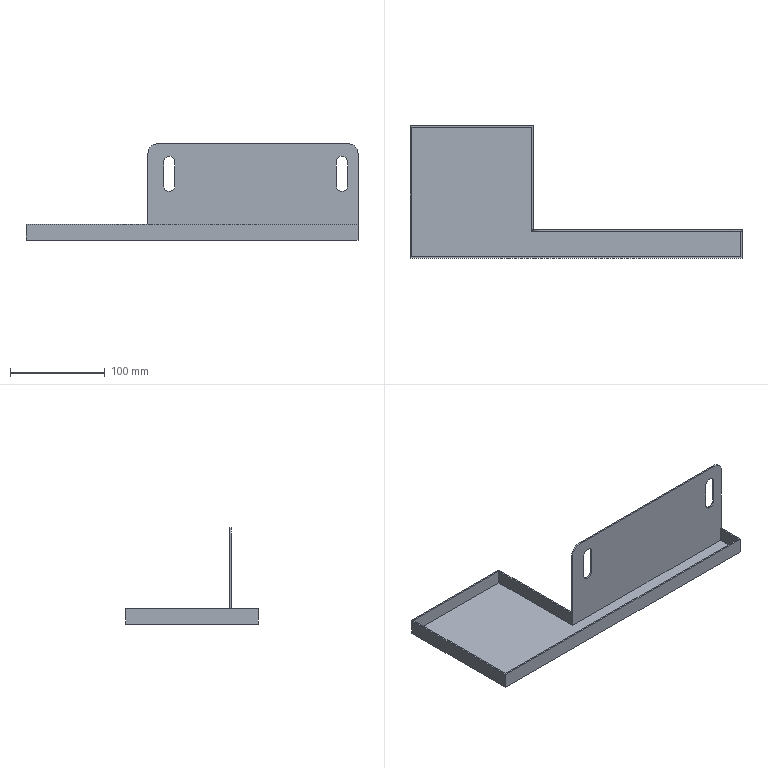Part | SolidWorks | features ICE 3, BossThin 1, Extrusion 1, Fillet 1 | 1 solid | 28 faces | box 350 x 140 x 101.5 mm | volume 86053 mm3 | plane 20 | cylinder 8 | commonest cylinder face diameters 12 x6 20 x2
STEP:
#1=CARTESIAN_POINT('',(-24.,-40.,51.5));
#2=VERTEX_POINT('',#1);
#3=CARTESIAN_POINT('',(-18.,-40.,57.5));
#4=VERTEX_POINT('',#3);
#5=CARTESIAN_POINT('',(-24.,-40.,57.5));
#6=DIRECTION('',(0.,-1.,0.));
#7=DIRECTION('',(1.,0.,0.));
#8=AXIS2_PLACEMENT_3D('',#5,#6,#7);
#9=CIRCLE('',#8,6.);
#10=EDGE_CURVE('',#2,#4,#9,.T.);
#11=ORIENTED_EDGE('',*,*,#10,.F.);
#12=CARTESIAN_POINT('',(-24.,-41.5,51.5));
#13=VERTEX_POINT('',#12);
#14=CARTESIAN_POINT('',(-24.,58.5,51.5));
#15=DIRECTION('',(0.,-1.,0.));
#16=VECTOR('',#15,1000.);
#17=LINE('',#14,#16);
#18=EDGE_CURVE('',#2,#13,#17,.T.);
#19=ORIENTED_EDGE('',*,*,#18,.T.);
#20=CARTESIAN_POINT('',(-18.,-41.5,57.5));
#21=VERTEX_POINT('',#20);
#22=CARTESIAN_POINT('',(-24.,-41.5,57.5));
#23=DIRECTION('',(0.,-1.,0.));
#24=DIRECTION('',(0.,0.,-1.));
#25=AXIS2_PLACEMENT_3D('',#22,#23,#24);
#26=CIRCLE('',#25,6.);
#27=EDGE_CURVE('',#13,#21,#26,.T.);
#28=ORIENTED_EDGE('',*,*,#27,.T.);
#29=CARTESIAN_POINT('',(-18.,58.5,57.5));
#30=DIRECTION('',(0.,-1.,0.));
#31=VECTOR('',#30,1000.);
#32=LINE('',#29,#31);
#33=EDGE_CURVE('',#4,#21,#32,.T.);
#34=ORIENTED_EDGE('',*,*,#33,.F.);
#35=EDGE_LOOP('',(#11,#19,#28,#34));
#36=FACE_OUTER_BOUND('',#35,.T.);
#37=CARTESIAN_POINT('',(-24.,58.5,57.5));
#38=DIRECTION('',(0.,-1.,0.));
#39=DIRECTION('',(0.,0.,-1.));
#40=AXIS2_PLACEMENT_3D('',#37,#38,#39);
#41=CYLINDRICAL_SURFACE('',#40,6.);
#42=ADVANCED_FACE('',(#36),#41,.F.);
#43=CARTESIAN_POINT('',(158.,-40.,51.5));
#44=VERTEX_POINT('',#43);
#45=CARTESIAN_POINT('',(164.,-40.,57.5));
#46=VERTEX_POINT('',#45);
#47=CARTESIAN_POINT('',(158.,-40.,57.5));
#48=DIRECTION('',(0.,-1.,0.));
#49=DIRECTION('',(1.,0.,0.));
#50=AXIS2_PLACEMENT_3D('',#47,#48,#49);
#51=CIRCLE('',#50,6.);
#52=EDGE_CURVE('',#44,#46,#51,.T.);
#53=ORIENTED_EDGE('',*,*,#52,.F.);
#54=CARTESIAN_POINT('',(158.,-41.5,51.5));
#55=VERTEX_POINT('',#54);
#56=CARTESIAN_POINT('',(158.,58.5,51.5));
#57=DIRECTION('',(0.,-1.,0.));
#58=VECTOR('',#57,1000.);
#59=LINE('',#56,#58);
#60=EDGE_CURVE('',#44,#55,#59,.T.);
#61=ORIENTED_EDGE('',*,*,#60,.T.);
#62=CARTESIAN_POINT('',(164.,-41.5,57.5));
#63=VERTEX_POINT('',#62);
#64=CARTESIAN_POINT('',(158.,-41.5,57.5));
#65=DIRECTION('',(0.,-1.,0.));
#66=DIRECTION('',(0.,0.,-1.));
#67=AXIS2_PLACEMENT_3D('',#64,#65,#66);
#68=CIRCLE('',#67,6.);
#69=EDGE_CURVE('',#55,#63,#68,.T.);
#70=ORIENTED_EDGE('',*,*,#69,.T.);
#71=CARTESIAN_POINT('',(164.,58.5,57.5));
#72=DIRECTION('',(0.,-1.,0.));
#73=VECTOR('',#72,1000.);
#74=LINE('',#71,#73);
#75=EDGE_CURVE('',#46,#63,#74,.T.);
#76=ORIENTED_EDGE('',*,*,#75,.F.);
#77=EDGE_LOOP('',(#53,#61,#70,#76));
#78=FACE_OUTER_BOUND('',#77,.T.);
#79=CARTESIAN_POINT('',(158.,58.5,57.5));
#80=DIRECTION('',(0.,-1.,0.));
#81=DIRECTION('',(0.,0.,-1.));
#82=AXIS2_PLACEMENT_3D('',#79,#80,#81);
#83=CYLINDRICAL_SURFACE('',#82,6.);
#84=ADVANCED_FACE('',(#78),#83,.F.);
#85=CARTESIAN_POINT('',(-46.5,-41.5,1.5));
#86=VERTEX_POINT('',#85);
#87=CARTESIAN_POINT('',(173.5,-41.5,1.5));
#88=VERTEX_POINT('',#87);
#89=CARTESIAN_POINT('',(-46.5,-41.5,1.5));
#90=DIRECTION('',(1.,0.,0.));
#91=VECTOR('',#90,1000.);
#92=LINE('',#89,#91);
#93=EDGE_CURVE('',#86,#88,#92,.T.);
#94=ORIENTED_EDGE('',*,*,#93,.F.);
#95=CARTESIAN_POINT('',(-46.5,68.5,1.5));
#96=VERTEX_POINT('',#95);
#97=CARTESIAN_POINT('',(-46.5,70.,1.5));
#98=DIRECTION('',(0.,1.,0.));
#99=VECTOR('',#98,1000.);
#100=LINE('',#97,#99);
#101=EDGE_CURVE('',#86,#96,#100,.T.);
#102=ORIENTED_EDGE('',*,*,#101,.T.);
#103=CARTESIAN_POINT('',(-173.5,68.5,1.5));
#104=VERTEX_POINT('',#103);
#105=CARTESIAN_POINT('',(-45.,68.5,1.5));
#106=DIRECTION('',(-1.,0.,0.));
#107=VECTOR('',#106,1000.);
#108=LINE('',#105,#107);
#109=EDGE_CURVE('',#96,#104,#108,.T.);
#110=ORIENTED_EDGE('',*,*,#109,.T.);
#111=CARTESIAN_POINT('',(-173.5,-68.5,1.5));
#112=VERTEX_POINT('',#111);
#113=CARTESIAN_POINT('',(-173.5,70.,1.5));
#114=DIRECTION('',(0.,-1.,0.));
#115=VECTOR('',#114,1000.);
#116=LINE('',#113,#115);
#117=EDGE_CURVE('',#104,#112,#116,.T.);
#118=ORIENTED_EDGE('',*,*,#117,.T.);
#119=CARTESIAN_POINT('',(173.5,-68.5,1.5));
#120=VERTEX_POINT('',#119);
#121=CARTESIAN_POINT('',(-175.,-68.5,1.5));
#122=DIRECTION('',(1.,0.,0.));
#123=VECTOR('',#122,1000.);
#124=LINE('',#121,#123);
#125=EDGE_CURVE('',#112,#120,#124,.T.);
#126=ORIENTED_EDGE('',*,*,#125,.T.);
#127=CARTESIAN_POINT('',(173.5,-70.,1.5));
#128=DIRECTION('',(0.,1.,0.));
#129=VECTOR('',#128,1000.);
#130=LINE('',#127,#129);
#131=EDGE_CURVE('',#120,#88,#130,.T.);
#132=ORIENTED_EDGE('',*,*,#131,.T.);
#133=EDGE_LOOP('',(#94,#102,#110,#118,#126,#132));
#134=FACE_OUTER_BOUND('',#133,.T.);
#135=CARTESIAN_POINT('',(0.,0.,1.5));
#136=DIRECTION('',(0.,0.,1.));
#137=DIRECTION('',(1.,0.,0.));
#138=AXIS2_PLACEMENT_3D('',#135,#136,#137);
#139=PLANE('',#138);
#140=ADVANCED_FACE('',(#134),#139,.T.);
#141=CARTESIAN_POINT('',(173.5,-68.5,16.5));
#142=VERTEX_POINT('',#141);
#143=CARTESIAN_POINT('',(173.5,-41.5,16.5));
#144=VERTEX_POINT('',#143);
#145=CARTESIAN_POINT('',(173.5,-70.,16.5));
#146=DIRECTION('',(0.,1.,0.));
#147=VECTOR('',#146,1000.);
#148=LINE('',#145,#147);
#149=EDGE_CURVE('',#142,#144,#148,.T.);
#150=ORIENTED_EDGE('',*,*,#149,.T.);
#151=CARTESIAN_POINT('',(173.5,-41.5,16.5));
#152=DIRECTION('',(0.,0.,-1.));
#153=VECTOR('',#152,1000.);
#154=LINE('',#151,#153);
#155=EDGE_CURVE('',#144,#88,#154,.T.);
#156=ORIENTED_EDGE('',*,*,#155,.T.);
#157=ORIENTED_EDGE('',*,*,#131,.F.);
#158=CARTESIAN_POINT('',(173.5,-68.5,16.5));
#159=DIRECTION('',(0.,0.,-1.));
#160=VECTOR('',#159,1000.);
#161=LINE('',#158,#160);
#162=EDGE_CURVE('',#142,#120,#161,.T.);
#163=ORIENTED_EDGE('',*,*,#162,.F.);
#164=EDGE_LOOP('',(#150,#156,#157,#163));
#165=FACE_OUTER_BOUND('',#164,.T.);
#166=CARTESIAN_POINT('',(173.5,-70.,16.5));
#167=DIRECTION('',(-1.,0.,0.));
#168=DIRECTION('',(0.,0.,1.));
#169=AXIS2_PLACEMENT_3D('',#166,#167,#168);
#170=PLANE('',#169);
#171=ADVANCED_FACE('',(#165),#170,.T.);
#172=CARTESIAN_POINT('',(175.,-41.5,16.5));
#173=VERTEX_POINT('',#172);
#174=CARTESIAN_POINT('',(0.,-41.5,16.5));
#175=DIRECTION('',(1.,0.,0.));
#176=VECTOR('',#175,1000.);
#177=LINE('',#174,#176);
#178=EDGE_CURVE('',#144,#173,#177,.T.);
#179=ORIENTED_EDGE('',*,*,#178,.F.);
#180=ORIENTED_EDGE('',*,*,#149,.F.);
#181=CARTESIAN_POINT('',(-173.5,-68.5,16.5));
#182=VERTEX_POINT('',#181);
#183=CARTESIAN_POINT('',(-175.,-68.5,16.5));
#184=DIRECTION('',(1.,0.,0.));
#185=VECTOR('',#184,1000.);
#186=LINE('',#183,#185);
#187=EDGE_CURVE('',#182,#142,#186,.T.);
#188=ORIENTED_EDGE('',*,*,#187,.F.);
#189=CARTESIAN_POINT('',(-173.5,68.5,16.5));
#190=VERTEX_POINT('',#189);
#191=CARTESIAN_POINT('',(-173.5,70.,16.5));
#192=DIRECTION('',(0.,-1.,0.));
#193=VECTOR('',#192,1000.);
#194=LINE('',#191,#193);
#195=EDGE_CURVE('',#190,#182,#194,.T.);
#196=ORIENTED_EDGE('',*,*,#195,.F.);
#197=CARTESIAN_POINT('',(-46.5,68.5,16.5));
#198=VERTEX_POINT('',#197);
#199=CARTESIAN_POINT('',(-45.,68.5,16.5));
#200=DIRECTION('',(-1.,0.,0.));
#201=VECTOR('',#200,1000.);
#202=LINE('',#199,#201);
#203=EDGE_CURVE('',#198,#190,#202,.T.);
#204=ORIENTED_EDGE('',*,*,#203,.F.);
#205=CARTESIAN_POINT('',(-46.5,-40.,16.5));
#206=VERTEX_POINT('',#205);
#207=CARTESIAN_POINT('',(-46.5,70.,16.5));
#208=DIRECTION('',(0.,1.,0.));
#209=VECTOR('',#208,1000.);
#210=LINE('',#207,#209);
#211=EDGE_CURVE('',#206,#198,#210,.T.);
#212=ORIENTED_EDGE('',*,*,#211,.F.);
#213=CARTESIAN_POINT('',(-45.,-40.,16.5));
#214=VERTEX_POINT('',#213);
#215=CARTESIAN_POINT('',(-45.,-40.,16.5));
#216=DIRECTION('',(-1.,0.,0.));
#217=VECTOR('',#216,1000.);
#218=LINE('',#215,#217);
#219=EDGE_CURVE('',#214,#206,#218,.T.);
#220=ORIENTED_EDGE('',*,*,#219,.F.);
#221=CARTESIAN_POINT('',(-45.,70.,16.5));
#222=VERTEX_POINT('',#221);
#223=CARTESIAN_POINT('',(-45.,70.,16.5));
#224=DIRECTION('',(0.,1.,0.));
#225=VECTOR('',#224,1000.);
#226=LINE('',#223,#225);
#227=EDGE_CURVE('',#214,#222,#226,.T.);
#228=ORIENTED_EDGE('',*,*,#227,.T.);
#229=CARTESIAN_POINT('',(-175.,70.,16.5));
#230=VERTEX_POINT('',#229);
#231=CARTESIAN_POINT('',(-45.,70.,16.5));
#232=DIRECTION('',(-1.,0.,0.));
#233=VECTOR('',#232,1000.);
#234=LINE('',#231,#233);
#235=EDGE_CURVE('',#222,#230,#234,.T.);
#236=ORIENTED_EDGE('',*,*,#235,.T.);
#237=CARTESIAN_POINT('',(-175.,-70.,16.5));
#238=VERTEX_POINT('',#237);
#239=CARTESIAN_POINT('',(-175.,70.,16.5));
#240=DIRECTION('',(0.,-1.,0.));
#241=VECTOR('',#240,1000.);
#242=LINE('',#239,#241);
#243=EDGE_CURVE('',#230,#238,#242,.T.);
#244=ORIENTED_EDGE('',*,*,#243,.T.);
#245=CARTESIAN_POINT('',(175.,-70.,16.5));
#246=VERTEX_POINT('',#245);
#247=CARTESIAN_POINT('',(-175.,-70.,16.5));
#248=DIRECTION('',(1.,0.,0.));
#249=VECTOR('',#248,1000.);
#250=LINE('',#247,#249);
#251=EDGE_CURVE('',#238,#246,#250,.T.);
#252=ORIENTED_EDGE('',*,*,#251,.T.);
#253=CARTESIAN_POINT('',(175.,-70.,16.5));
#254=DIRECTION('',(0.,1.,0.));
#255=VECTOR('',#254,1000.);
#256=LINE('',#253,#255);
#257=EDGE_CURVE('',#246,#173,#256,.T.);
#258=ORIENTED_EDGE('',*,*,#257,.T.);
#259=EDGE_LOOP('',(#179,#180,#188,#196,#204,#212,#220,#228,#236,#244,#252,#258));
#260=FACE_OUTER_BOUND('',#259,.T.);
#261=CARTESIAN_POINT('',(0.,0.,16.5));
#262=DIRECTION('',(0.,0.,-1.));
#263=DIRECTION('',(-1.,0.,0.));
#264=AXIS2_PLACEMENT_3D('',#261,#262,#263);
#265=PLANE('',#264);
#266=ADVANCED_FACE('',(#260),#265,.F.);
#267=CARTESIAN_POINT('',(175.,-40.,0.));
#268=VERTEX_POINT('',#267);
#269=CARTESIAN_POINT('',(175.,-40.,91.5));
#270=VERTEX_POINT('',#269);
#271=CARTESIAN_POINT('',(175.,-40.,-0.5));
#272=DIRECTION('',(0.,0.,1.));
#273=VECTOR('',#272,1000.);
#274=LINE('',#271,#273);
#275=EDGE_CURVE('',#268,#270,#274,.T.);
#276=ORIENTED_EDGE('',*,*,#275,.T.);
#277=CARTESIAN_POINT('',(175.,-41.5,91.5));
#278=VERTEX_POINT('',#277);
#279=CARTESIAN_POINT('',(175.,-41.5,91.5));
#280=DIRECTION('',(0.,-1.,0.));
#281=VECTOR('',#280,1000.);
#282=LINE('',#279,#281);
#283=EDGE_CURVE('',#270,#278,#282,.T.);
#284=ORIENTED_EDGE('',*,*,#283,.T.);
#285=CARTESIAN_POINT('',(175.,-41.5,101.5));
#286=DIRECTION('',(0.,0.,-1.));
#287=VECTOR('',#286,1000.);
#288=LINE('',#285,#287);
#289=EDGE_CURVE('',#278,#173,#288,.T.);
#290=ORIENTED_EDGE('',*,*,#289,.T.);
#291=ORIENTED_EDGE('',*,*,#257,.F.);
#292=CARTESIAN_POINT('',(175.,-70.,0.));
#293=VERTEX_POINT('',#292);
#294=CARTESIAN_POINT('',(175.,-70.,1.5));
#295=DIRECTION('',(0.,0.,-1.));
#296=VECTOR('',#295,1000.);
#297=LINE('',#294,#296);
#298=EDGE_CURVE('',#246,#293,#297,.T.);
#299=ORIENTED_EDGE('',*,*,#298,.T.);
#300=CARTESIAN_POINT('',(175.,70.,0.));
#301=DIRECTION('',(0.,1.,0.));
#302=VECTOR('',#301,1000.);
#303=LINE('',#300,#302);
#304=EDGE_CURVE('',#293,#268,#303,.T.);
#305=ORIENTED_EDGE('',*,*,#304,.T.);
#306=EDGE_LOOP('',(#276,#284,#290,#291,#299,#305));
#307=FACE_OUTER_BOUND('',#306,.T.);
#308=CARTESIAN_POINT('',(175.,70.,1.5));
#309=DIRECTION('',(-1.,0.,0.));
#310=DIRECTION('',(0.,0.,1.));
#311=AXIS2_PLACEMENT_3D('',#308,#309,#310);
#312=PLANE('',#311);
#313=ADVANCED_FACE('',(#307),#312,.F.);
#314=CARTESIAN_POINT('',(-175.,70.,0.));
#315=VERTEX_POINT('',#314);
#316=CARTESIAN_POINT('',(-175.,70.,1.5));
#317=DIRECTION('',(0.,0.,-1.));
#318=VECTOR('',#317,1000.);
#319=LINE('',#316,#318);
#320=EDGE_CURVE('',#230,#315,#319,.T.);
#321=ORIENTED_EDGE('',*,*,#320,.F.);
#322=ORIENTED_EDGE('',*,*,#235,.F.);
#323=CARTESIAN_POINT('',(-45.,70.,0.));
#324=VERTEX_POINT('',#323);
#325=CARTESIAN_POINT('',(-45.,70.,-0.5));
#326=DIRECTION('',(0.,0.,1.));
#327=VECTOR('',#326,1000.);
#328=LINE('',#325,#327);
#329=EDGE_CURVE('',#324,#222,#328,.T.);
#330=ORIENTED_EDGE('',*,*,#329,.F.);
#331=CARTESIAN_POINT('',(-175.,70.,0.));
#332=DIRECTION('',(-1.,0.,0.));
#333=VECTOR('',#332,1000.);
#334=LINE('',#331,#333);
#335=EDGE_CURVE('',#324,#315,#334,.T.);
#336=ORIENTED_EDGE('',*,*,#335,.T.);
#337=EDGE_LOOP('',(#321,#322,#330,#336));
#338=FACE_OUTER_BOUND('',#337,.T.);
#339=CARTESIAN_POINT('',(-175.,70.,1.5));
#340=DIRECTION('',(0.,-1.,0.));
#341=DIRECTION('',(0.,0.,-1.));
#342=AXIS2_PLACEMENT_3D('',#339,#340,#341);
#343=PLANE('',#342);
#344=ADVANCED_FACE('',(#338),#343,.F.);
#345=CARTESIAN_POINT('',(-175.,-70.,0.));
#346=VERTEX_POINT('',#345);
#347=CARTESIAN_POINT('',(-175.,70.,0.));
#348=DIRECTION('',(0.,-1.,0.));
#349=VECTOR('',#348,1000.);
#350=LINE('',#347,#349);
#351=EDGE_CURVE('',#315,#346,#350,.T.);
#352=ORIENTED_EDGE('',*,*,#351,.T.);
#353=CARTESIAN_POINT('',(-175.,-70.,1.5));
#354=DIRECTION('',(0.,0.,-1.));
#355=VECTOR('',#354,1000.);
#356=LINE('',#353,#355);
#357=EDGE_CURVE('',#238,#346,#356,.T.);
#358=ORIENTED_EDGE('',*,*,#357,.F.);
#359=ORIENTED_EDGE('',*,*,#243,.F.);
#360=ORIENTED_EDGE('',*,*,#320,.T.);
#361=EDGE_LOOP('',(#352,#358,#359,#360));
#362=FACE_OUTER_BOUND('',#361,.T.);
#363=CARTESIAN_POINT('',(-175.,70.,1.5));
#364=DIRECTION('',(1.,0.,0.));
#365=DIRECTION('',(0.,0.,-1.));
#366=AXIS2_PLACEMENT_3D('',#363,#364,#365);
#367=PLANE('',#366);
#368=ADVANCED_FACE('',(#362),#367,.F.);
#369=CARTESIAN_POINT('',(-175.,-70.,0.));
#370=DIRECTION('',(1.,0.,0.));
#371=VECTOR('',#370,1000.);
#372=LINE('',#369,#371);
#373=EDGE_CURVE('',#346,#293,#372,.T.);
#374=ORIENTED_EDGE('',*,*,#373,.T.);
#375=ORIENTED_EDGE('',*,*,#298,.F.);
#376=ORIENTED_EDGE('',*,*,#251,.F.);
#377=ORIENTED_EDGE('',*,*,#357,.T.);
#378=EDGE_LOOP('',(#374,#375,#376,#377));
#379=FACE_OUTER_BOUND('',#378,.T.);
#380=CARTESIAN_POINT('',(-175.,-70.,1.5));
#381=DIRECTION('',(0.,1.,0.));
#382=DIRECTION('',(0.,0.,1.));
#383=AXIS2_PLACEMENT_3D('',#380,#381,#382);
#384=PLANE('',#383);
#385=ADVANCED_FACE('',(#379),#384,.F.);
#386=CARTESIAN_POINT('',(-45.,-40.,0.));
#387=VERTEX_POINT('',#386);
#388=CARTESIAN_POINT('',(-45.,0.,0.));
#389=DIRECTION('',(0.,-1.,0.));
#390=VECTOR('',#389,1000.);
#391=LINE('',#388,#390);
#392=EDGE_CURVE('',#324,#387,#391,.T.);
#393=ORIENTED_EDGE('',*,*,#392,.T.);
#394=CARTESIAN_POINT('',(0.,-40.,0.));
#395=DIRECTION('',(1.,0.,0.));
#396=VECTOR('',#395,1000.);
#397=LINE('',#394,#396);
#398=EDGE_CURVE('',#387,#268,#397,.T.);
#399=ORIENTED_EDGE('',*,*,#398,.T.);
#400=ORIENTED_EDGE('',*,*,#304,.F.);
#401=ORIENTED_EDGE('',*,*,#373,.F.);
#402=ORIENTED_EDGE('',*,*,#351,.F.);
#403=ORIENTED_EDGE('',*,*,#335,.F.);
#404=EDGE_LOOP('',(#393,#399,#400,#401,#402,#403));
#405=FACE_OUTER_BOUND('',#404,.T.);
#406=CARTESIAN_POINT('',(0.,0.,0.));
#407=DIRECTION('',(0.,0.,1.));
#408=DIRECTION('',(1.,0.,0.));
#409=AXIS2_PLACEMENT_3D('',#406,#407,#408);
#410=PLANE('',#409);
#411=ADVANCED_FACE('',(#405),#410,.F.);
#412=CARTESIAN_POINT('',(-18.,-40.,82.5));
#413=VERTEX_POINT('',#412);
#414=CARTESIAN_POINT('',(-18.,-40.,-0.5));
#415=DIRECTION('',(0.,0.,1.));
#416=VECTOR('',#415,1000.);
#417=LINE('',#414,#416);
#418=EDGE_CURVE('',#4,#413,#417,.T.);
#419=ORIENTED_EDGE('',*,*,#418,.T.);
#420=CARTESIAN_POINT('',(-30.,-40.,82.5));
#421=VERTEX_POINT('',#420);
#422=CARTESIAN_POINT('',(-24.,-40.,82.5));
#423=DIRECTION('',(0.,-1.,0.));
#424=DIRECTION('',(1.,0.,0.));
#425=AXIS2_PLACEMENT_3D('',#422,#423,#424);
#426=CIRCLE('',#425,6.);
#427=EDGE_CURVE('',#413,#421,#426,.T.);
#428=ORIENTED_EDGE('',*,*,#427,.T.);
#429=CARTESIAN_POINT('',(-30.,-40.,57.5));
#430=VERTEX_POINT('',#429);
#431=CARTESIAN_POINT('',(-30.,-40.,-0.5));
#432=DIRECTION('',(0.,0.,-1.));
#433=VECTOR('',#432,1000.);
#434=LINE('',#431,#433);
#435=EDGE_CURVE('',#421,#430,#434,.T.);
#436=ORIENTED_EDGE('',*,*,#435,.T.);
#437=CARTESIAN_POINT('',(-24.,-40.,57.5));
#438=DIRECTION('',(0.,-1.,0.));
#439=DIRECTION('',(1.,0.,0.));
#440=AXIS2_PLACEMENT_3D('',#437,#438,#439);
#441=CIRCLE('',#440,6.);
#442=EDGE_CURVE('',#430,#2,#441,.T.);
#443=ORIENTED_EDGE('',*,*,#442,.T.);
#444=ORIENTED_EDGE('',*,*,#10,.T.);
#445=EDGE_LOOP('',(#419,#428,#436,#443,#444));
#446=FACE_BOUND('',#445,.T.);
#447=CARTESIAN_POINT('',(164.,-40.,82.5));
#448=VERTEX_POINT('',#447);
#449=CARTESIAN_POINT('',(164.,-40.,-0.5));
#450=DIRECTION('',(0.,0.,1.));
#451=VECTOR('',#450,1000.);
#452=LINE('',#449,#451);
#453=EDGE_CURVE('',#46,#448,#452,.T.);
#454=ORIENTED_EDGE('',*,*,#453,.T.);
#455=CARTESIAN_POINT('',(152.,-40.,82.5));
#456=VERTEX_POINT('',#455);
#457=CARTESIAN_POINT('',(158.,-40.,82.5));
#458=DIRECTION('',(0.,-1.,0.));
#459=DIRECTION('',(1.,0.,0.));
#460=AXIS2_PLACEMENT_3D('',#457,#458,#459);
#461=CIRCLE('',#460,6.);
#462=EDGE_CURVE('',#448,#456,#461,.T.);
#463=ORIENTED_EDGE('',*,*,#462,.T.);
#464=CARTESIAN_POINT('',(152.,-40.,57.5));
#465=VERTEX_POINT('',#464);
#466=CARTESIAN_POINT('',(152.,-40.,-0.5));
#467=DIRECTION('',(0.,0.,-1.));
#468=VECTOR('',#467,1000.);
#469=LINE('',#466,#468);
#470=EDGE_CURVE('',#456,#465,#469,.T.);
#471=ORIENTED_EDGE('',*,*,#470,.T.);
#472=CARTESIAN_POINT('',(158.,-40.,57.5));
#473=DIRECTION('',(0.,-1.,0.));
#474=DIRECTION('',(1.,0.,0.));
#475=AXIS2_PLACEMENT_3D('',#472,#473,#474);
#476=CIRCLE('',#475,6.);
#477=EDGE_CURVE('',#465,#44,#476,.T.);
#478=ORIENTED_EDGE('',*,*,#477,.T.);
#479=ORIENTED_EDGE('',*,*,#52,.T.);
#480=EDGE_LOOP('',(#454,#463,#471,#478,#479));
#481=FACE_BOUND('',#480,.T.);
#482=CARTESIAN_POINT('',(165.,-40.,101.5));
#483=VERTEX_POINT('',#482);
#484=CARTESIAN_POINT('',(-36.5,-40.,101.5));
#485=VERTEX_POINT('',#484);
#486=CARTESIAN_POINT('',(-46.5,-40.,101.5));
#487=DIRECTION('',(-1.,0.,0.));
#488=VECTOR('',#487,1000.);
#489=LINE('',#486,#488);
#490=EDGE_CURVE('',#483,#485,#489,.T.);
#491=ORIENTED_EDGE('',*,*,#490,.F.);
#492=CARTESIAN_POINT('',(165.,-40.,91.5));
#493=DIRECTION('',(0.,1.,0.));
#494=DIRECTION('',(1.,0.,0.));
#495=AXIS2_PLACEMENT_3D('',#492,#493,#494);
#496=CIRCLE('',#495,10.);
#497=EDGE_CURVE('',#483,#270,#496,.T.);
#498=ORIENTED_EDGE('',*,*,#497,.T.);
#499=ORIENTED_EDGE('',*,*,#275,.F.);
#500=ORIENTED_EDGE('',*,*,#398,.F.);
#501=CARTESIAN_POINT('',(-45.,-40.,-0.5));
#502=DIRECTION('',(0.,0.,1.));
#503=VECTOR('',#502,1000.);
#504=LINE('',#501,#503);
#505=EDGE_CURVE('',#387,#214,#504,.T.);
#506=ORIENTED_EDGE('',*,*,#505,.T.);
#507=ORIENTED_EDGE('',*,*,#219,.T.);
#508=CARTESIAN_POINT('',(-46.5,-40.,91.5));
#509=VERTEX_POINT('',#508);
#510=CARTESIAN_POINT('',(-46.5,-40.,101.5));
#511=DIRECTION('',(0.,0.,-1.));
#512=VECTOR('',#511,1000.);
#513=LINE('',#510,#512);
#514=EDGE_CURVE('',#509,#206,#513,.T.);
#515=ORIENTED_EDGE('',*,*,#514,.F.);
#516=CARTESIAN_POINT('',(-36.5,-40.,91.5));
#517=DIRECTION('',(0.,1.,0.));
#518=DIRECTION('',(1.,0.,0.));
#519=AXIS2_PLACEMENT_3D('',#516,#517,#518);
#520=CIRCLE('',#519,10.);
#521=EDGE_CURVE('',#509,#485,#520,.T.);
#522=ORIENTED_EDGE('',*,*,#521,.T.);
#523=EDGE_LOOP('',(#491,#498,#499,#500,#506,#507,#515,#522));
#524=FACE_OUTER_BOUND('',#523,.T.);
#525=CARTESIAN_POINT('',(175.,-40.,-0.5));
#526=DIRECTION('',(0.,-1.,0.));
#527=DIRECTION('',(1.,0.,0.));
#528=AXIS2_PLACEMENT_3D('',#525,#526,#527);
#529=PLANE('',#528);
#530=ADVANCED_FACE('',(#446,#481,#524),#529,.F.);
#531=ORIENTED_EDGE('',*,*,#329,.T.);
#532=ORIENTED_EDGE('',*,*,#227,.F.);
#533=ORIENTED_EDGE('',*,*,#505,.F.);
#534=ORIENTED_EDGE('',*,*,#392,.F.);
#535=EDGE_LOOP('',(#531,#532,#533,#534));
#536=FACE_OUTER_BOUND('',#535,.T.);
#537=CARTESIAN_POINT('',(-45.,70.,-0.5));
#538=DIRECTION('',(-1.,0.,0.));
#539=DIRECTION('',(0.,-1.,0.));
#540=AXIS2_PLACEMENT_3D('',#537,#538,#539);
#541=PLANE('',#540);
#542=ADVANCED_FACE('',(#536),#541,.F.);
#543=ORIENTED_EDGE('',*,*,#125,.F.);
#544=CARTESIAN_POINT('',(-173.5,-68.5,16.5));
#545=DIRECTION('',(0.,0.,-1.));
#546=VECTOR('',#545,1000.);
#547=LINE('',#544,#546);
#548=EDGE_CURVE('',#182,#112,#547,.T.);
#549=ORIENTED_EDGE('',*,*,#548,.F.);
#550=ORIENTED_EDGE('',*,*,#187,.T.);
#551=ORIENTED_EDGE('',*,*,#162,.T.);
#552=EDGE_LOOP('',(#543,#549,#550,#551));
#553=FACE_OUTER_BOUND('',#552,.T.);
#554=CARTESIAN_POINT('',(-175.,-68.5,16.5));
#555=DIRECTION('',(0.,1.,0.));
#556=DIRECTION('',(0.,0.,1.));
#557=AXIS2_PLACEMENT_3D('',#554,#555,#556);
#558=PLANE('',#557);
#559=ADVANCED_FACE('',(#553),#558,.T.);
#560=ORIENTED_EDGE('',*,*,#117,.F.);
#561=CARTESIAN_POINT('',(-173.5,68.5,16.5));
#562=DIRECTION('',(0.,0.,-1.));
#563=VECTOR('',#562,1000.);
#564=LINE('',#561,#563);
#565=EDGE_CURVE('',#190,#104,#564,.T.);
#566=ORIENTED_EDGE('',*,*,#565,.F.);
#567=ORIENTED_EDGE('',*,*,#195,.T.);
#568=ORIENTED_EDGE('',*,*,#548,.T.);
#569=EDGE_LOOP('',(#560,#566,#567,#568));
#570=FACE_OUTER_BOUND('',#569,.T.);
#571=CARTESIAN_POINT('',(-173.5,70.,16.5));
#572=DIRECTION('',(1.,0.,0.));
#573=DIRECTION('',(0.,0.,-1.));
#574=AXIS2_PLACEMENT_3D('',#571,#572,#573);
#575=PLANE('',#574);
#576=ADVANCED_FACE('',(#570),#575,.T.);
#577=ORIENTED_EDGE('',*,*,#109,.F.);
#578=CARTESIAN_POINT('',(-46.5,68.5,16.5));
#579=DIRECTION('',(0.,0.,-1.));
#580=VECTOR('',#579,1000.);
#581=LINE('',#578,#580);
#582=EDGE_CURVE('',#198,#96,#581,.T.);
#583=ORIENTED_EDGE('',*,*,#582,.F.);
#584=ORIENTED_EDGE('',*,*,#203,.T.);
#585=ORIENTED_EDGE('',*,*,#565,.T.);
#586=EDGE_LOOP('',(#577,#583,#584,#585));
#587=FACE_OUTER_BOUND('',#586,.T.);
#588=CARTESIAN_POINT('',(-45.,68.5,16.5));
#589=DIRECTION('',(0.,-1.,0.));
#590=DIRECTION('',(1.,0.,0.));
#591=AXIS2_PLACEMENT_3D('',#588,#589,#590);
#592=PLANE('',#591);
#593=ADVANCED_FACE('',(#587),#592,.T.);
#594=CARTESIAN_POINT('',(-46.5,-41.5,91.5));
#595=VERTEX_POINT('',#594);
#596=CARTESIAN_POINT('',(-46.5,-41.5,101.5));
#597=DIRECTION('',(0.,0.,-1.));
#598=VECTOR('',#597,1000.);
#599=LINE('',#596,#598);
#600=EDGE_CURVE('',#595,#86,#599,.T.);
#601=ORIENTED_EDGE('',*,*,#600,.F.);
#602=CARTESIAN_POINT('',(-46.5,70.,91.5));
#603=DIRECTION('',(0.,1.,0.));
#604=VECTOR('',#603,1000.);
#605=LINE('',#602,#604);
#606=EDGE_CURVE('',#595,#509,#605,.T.);
#607=ORIENTED_EDGE('',*,*,#606,.T.);
#608=ORIENTED_EDGE('',*,*,#514,.T.);
#609=ORIENTED_EDGE('',*,*,#211,.T.);
#610=ORIENTED_EDGE('',*,*,#582,.T.);
#611=ORIENTED_EDGE('',*,*,#101,.F.);
#612=EDGE_LOOP('',(#601,#607,#608,#609,#610,#611));
#613=FACE_OUTER_BOUND('',#612,.T.);
#614=CARTESIAN_POINT('',(-46.5,70.,16.5));
#615=DIRECTION('',(-1.,0.,0.));
#616=DIRECTION('',(0.,-1.,0.));
#617=AXIS2_PLACEMENT_3D('',#614,#615,#616);
#618=PLANE('',#617);
#619=ADVANCED_FACE('',(#613),#618,.T.);
#620=CARTESIAN_POINT('',(-30.,-41.5,82.5));
#621=VERTEX_POINT('',#620);
#622=CARTESIAN_POINT('',(-30.,-41.5,57.5));
#623=VERTEX_POINT('',#622);
#624=CARTESIAN_POINT('',(-30.,-41.5,82.5));
#625=DIRECTION('',(0.,0.,-1.));
#626=VECTOR('',#625,1000.);
#627=LINE('',#624,#626);
#628=EDGE_CURVE('',#621,#623,#627,.T.);
#629=ORIENTED_EDGE('',*,*,#628,.F.);
#630=CARTESIAN_POINT('',(-18.,-41.5,82.5));
#631=VERTEX_POINT('',#630);
#632=CARTESIAN_POINT('',(-24.,-41.5,82.5));
#633=DIRECTION('',(0.,-1.,0.));
#634=DIRECTION('',(0.,0.,-1.));
#635=AXIS2_PLACEMENT_3D('',#632,#633,#634);
#636=CIRCLE('',#635,6.);
#637=EDGE_CURVE('',#631,#621,#636,.T.);
#638=ORIENTED_EDGE('',*,*,#637,.F.);
#639=CARTESIAN_POINT('',(-18.,-41.5,82.5));
#640=DIRECTION('',(0.,0.,1.));
#641=VECTOR('',#640,1000.);
#642=LINE('',#639,#641);
#643=EDGE_CURVE('',#21,#631,#642,.T.);
#644=ORIENTED_EDGE('',*,*,#643,.F.);
#645=ORIENTED_EDGE('',*,*,#27,.F.);
#646=CARTESIAN_POINT('',(-24.,-41.5,57.5));
#647=DIRECTION('',(0.,-1.,0.));
#648=DIRECTION('',(0.,0.,-1.));
#649=AXIS2_PLACEMENT_3D('',#646,#647,#648);
#650=CIRCLE('',#649,6.);
#651=EDGE_CURVE('',#623,#13,#650,.T.);
#652=ORIENTED_EDGE('',*,*,#651,.F.);
#653=EDGE_LOOP('',(#629,#638,#644,#645,#652));
#654=FACE_BOUND('',#653,.T.);
#655=CARTESIAN_POINT('',(152.,-41.5,82.5));
#656=VERTEX_POINT('',#655);
#657=CARTESIAN_POINT('',(152.,-41.5,57.5));
#658=VERTEX_POINT('',#657);
#659=CARTESIAN_POINT('',(152.,-41.5,82.5));
#660=DIRECTION('',(0.,0.,-1.));
#661=VECTOR('',#660,1000.);
#662=LINE('',#659,#661);
#663=EDGE_CURVE('',#656,#658,#662,.T.);
#664=ORIENTED_EDGE('',*,*,#663,.F.);
#665=CARTESIAN_POINT('',(164.,-41.5,82.5));
#666=VERTEX_POINT('',#665);
#667=CARTESIAN_POINT('',(158.,-41.5,82.5));
#668=DIRECTION('',(0.,-1.,0.));
#669=DIRECTION('',(0.,0.,-1.));
#670=AXIS2_PLACEMENT_3D('',#667,#668,#669);
#671=CIRCLE('',#670,6.);
#672=EDGE_CURVE('',#666,#656,#671,.T.);
#673=ORIENTED_EDGE('',*,*,#672,.F.);
#674=CARTESIAN_POINT('',(164.,-41.5,82.5));
#675=DIRECTION('',(0.,0.,1.));
#676=VECTOR('',#675,1000.);
#677=LINE('',#674,#676);
#678=EDGE_CURVE('',#63,#666,#677,.T.);
#679=ORIENTED_EDGE('',*,*,#678,.F.);
#680=ORIENTED_EDGE('',*,*,#69,.F.);
#681=CARTESIAN_POINT('',(158.,-41.5,57.5));
#682=DIRECTION('',(0.,-1.,0.));
#683=DIRECTION('',(0.,0.,-1.));
#684=AXIS2_PLACEMENT_3D('',#681,#682,#683);
#685=CIRCLE('',#684,6.);
#686=EDGE_CURVE('',#658,#55,#685,.T.);
#687=ORIENTED_EDGE('',*,*,#686,.F.);
#688=EDGE_LOOP('',(#664,#673,#679,#680,#687));
#689=FACE_BOUND('',#688,.T.);
#690=ORIENTED_EDGE('',*,*,#289,.F.);
#691=CARTESIAN_POINT('',(165.,-41.5,101.5));
#692=VERTEX_POINT('',#691);
#693=CARTESIAN_POINT('',(165.,-41.5,91.5));
#694=DIRECTION('',(0.,-1.,0.));
#695=DIRECTION('',(0.,0.,1.));
#696=AXIS2_PLACEMENT_3D('',#693,#694,#695);
#697=CIRCLE('',#696,10.);
#698=EDGE_CURVE('',#278,#692,#697,.T.);
#699=ORIENTED_EDGE('',*,*,#698,.T.);
#700=CARTESIAN_POINT('',(-36.5,-41.5,101.5));
#701=VERTEX_POINT('',#700);
#702=CARTESIAN_POINT('',(-46.5,-41.5,101.5));
#703=DIRECTION('',(1.,0.,0.));
#704=VECTOR('',#703,1000.);
#705=LINE('',#702,#704);
#706=EDGE_CURVE('',#701,#692,#705,.T.);
#707=ORIENTED_EDGE('',*,*,#706,.F.);
#708=CARTESIAN_POINT('',(-36.5,-41.5,91.5));
#709=DIRECTION('',(0.,-1.,0.));
#710=DIRECTION('',(0.,0.,1.));
#711=AXIS2_PLACEMENT_3D('',#708,#709,#710);
#712=CIRCLE('',#711,10.);
#713=EDGE_CURVE('',#701,#595,#712,.T.);
#714=ORIENTED_EDGE('',*,*,#713,.T.);
#715=ORIENTED_EDGE('',*,*,#600,.T.);
#716=ORIENTED_EDGE('',*,*,#93,.T.);
#717=ORIENTED_EDGE('',*,*,#155,.F.);
#718=ORIENTED_EDGE('',*,*,#178,.T.);
#719=EDGE_LOOP('',(#690,#699,#707,#714,#715,#716,#717,#718));
#720=FACE_OUTER_BOUND('',#719,.T.);
#721=CARTESIAN_POINT('',(-46.5,-41.5,101.5));
#722=DIRECTION('',(0.,1.,0.));
#723=DIRECTION('',(0.,0.,1.));
#724=AXIS2_PLACEMENT_3D('',#721,#722,#723);
#725=PLANE('',#724);
#726=ADVANCED_FACE('',(#654,#689,#720),#725,.F.);
#727=ORIENTED_EDGE('',*,*,#706,.T.);
#728=CARTESIAN_POINT('',(165.,-40.,101.5));
#729=DIRECTION('',(0.,1.,0.));
#730=VECTOR('',#729,1000.);
#731=LINE('',#728,#730);
#732=EDGE_CURVE('',#692,#483,#731,.T.);
#733=ORIENTED_EDGE('',*,*,#732,.T.);
#734=ORIENTED_EDGE('',*,*,#490,.T.);
#735=CARTESIAN_POINT('',(-36.5,0.,101.5));
#736=DIRECTION('',(0.,-1.,0.));
#737=VECTOR('',#736,1000.);
#738=LINE('',#735,#737);
#739=EDGE_CURVE('',#485,#701,#738,.T.);
#740=ORIENTED_EDGE('',*,*,#739,.T.);
#741=EDGE_LOOP('',(#727,#733,#734,#740));
#742=FACE_OUTER_BOUND('',#741,.T.);
#743=CARTESIAN_POINT('',(0.,0.,101.5));
#744=DIRECTION('',(0.,0.,1.));
#745=DIRECTION('',(1.,0.,0.));
#746=AXIS2_PLACEMENT_3D('',#743,#744,#745);
#747=PLANE('',#746);
#748=ADVANCED_FACE('',(#742),#747,.T.);
#749=ORIENTED_EDGE('',*,*,#698,.F.);
#750=ORIENTED_EDGE('',*,*,#283,.F.);
#751=ORIENTED_EDGE('',*,*,#497,.F.);
#752=ORIENTED_EDGE('',*,*,#732,.F.);
#753=EDGE_LOOP('',(#749,#750,#751,#752));
#754=FACE_OUTER_BOUND('',#753,.T.);
#755=CARTESIAN_POINT('',(165.,0.,91.5));
#756=DIRECTION('',(0.,-1.,0.));
#757=DIRECTION('',(0.,0.,-1.));
#758=AXIS2_PLACEMENT_3D('',#755,#756,#757);
#759=CYLINDRICAL_SURFACE('',#758,10.);
#760=ADVANCED_FACE('',(#754),#759,.T.);
#761=ORIENTED_EDGE('',*,*,#521,.F.);
#762=ORIENTED_EDGE('',*,*,#606,.F.);
#763=ORIENTED_EDGE('',*,*,#713,.F.);
#764=ORIENTED_EDGE('',*,*,#739,.F.);
#765=EDGE_LOOP('',(#761,#762,#763,#764));
#766=FACE_OUTER_BOUND('',#765,.T.);
#767=CARTESIAN_POINT('',(-36.5,0.,91.5));
#768=DIRECTION('',(0.,-1.,0.));
#769=DIRECTION('',(1.,0.,0.));
#770=AXIS2_PLACEMENT_3D('',#767,#768,#769);
#771=CYLINDRICAL_SURFACE('',#770,10.);
#772=ADVANCED_FACE('',(#766),#771,.T.);
#773=CARTESIAN_POINT('',(164.,58.5,82.5));
#774=DIRECTION('',(0.,-1.,0.));
#775=VECTOR('',#774,1000.);
#776=LINE('',#773,#775);
#777=EDGE_CURVE('',#448,#666,#776,.T.);
#778=ORIENTED_EDGE('',*,*,#777,.T.);
#779=ORIENTED_EDGE('',*,*,#672,.T.);
#780=CARTESIAN_POINT('',(152.,58.5,82.5));
#781=DIRECTION('',(0.,-1.,0.));
#782=VECTOR('',#781,1000.);
#783=LINE('',#780,#782);
#784=EDGE_CURVE('',#456,#656,#783,.T.);
#785=ORIENTED_EDGE('',*,*,#784,.F.);
#786=ORIENTED_EDGE('',*,*,#462,.F.);
#787=EDGE_LOOP('',(#778,#779,#785,#786));
#788=FACE_OUTER_BOUND('',#787,.T.);
#789=CARTESIAN_POINT('',(158.,58.5,82.5));
#790=DIRECTION('',(0.,-1.,0.));
#791=DIRECTION('',(0.,0.,-1.));
#792=AXIS2_PLACEMENT_3D('',#789,#790,#791);
#793=CYLINDRICAL_SURFACE('',#792,6.);
#794=ADVANCED_FACE('',(#788),#793,.F.);
#795=ORIENTED_EDGE('',*,*,#75,.T.);
#796=ORIENTED_EDGE('',*,*,#678,.T.);
#797=ORIENTED_EDGE('',*,*,#777,.F.);
#798=ORIENTED_EDGE('',*,*,#453,.F.);
#799=EDGE_LOOP('',(#795,#796,#797,#798));
#800=FACE_OUTER_BOUND('',#799,.T.);
#801=CARTESIAN_POINT('',(164.,58.5,82.5));
#802=DIRECTION('',(1.,0.,0.));
#803=DIRECTION('',(0.,0.,-1.));
#804=AXIS2_PLACEMENT_3D('',#801,#802,#803);
#805=PLANE('',#804);
#806=ADVANCED_FACE('',(#800),#805,.F.);
#807=ORIENTED_EDGE('',*,*,#60,.F.);
#808=ORIENTED_EDGE('',*,*,#477,.F.);
#809=CARTESIAN_POINT('',(152.,58.5,57.5));
#810=DIRECTION('',(0.,-1.,0.));
#811=VECTOR('',#810,1000.);
#812=LINE('',#809,#811);
#813=EDGE_CURVE('',#465,#658,#812,.T.);
#814=ORIENTED_EDGE('',*,*,#813,.T.);
#815=ORIENTED_EDGE('',*,*,#686,.T.);
#816=EDGE_LOOP('',(#807,#808,#814,#815));
#817=FACE_OUTER_BOUND('',#816,.T.);
#818=CARTESIAN_POINT('',(158.,58.5,57.5));
#819=DIRECTION('',(0.,-1.,0.));
#820=DIRECTION('',(0.,0.,-1.));
#821=AXIS2_PLACEMENT_3D('',#818,#819,#820);
#822=CYLINDRICAL_SURFACE('',#821,6.);
#823=ADVANCED_FACE('',(#817),#822,.F.);
#824=ORIENTED_EDGE('',*,*,#784,.T.);
#825=ORIENTED_EDGE('',*,*,#663,.T.);
#826=ORIENTED_EDGE('',*,*,#813,.F.);
#827=ORIENTED_EDGE('',*,*,#470,.F.);
#828=EDGE_LOOP('',(#824,#825,#826,#827));
#829=FACE_OUTER_BOUND('',#828,.T.);
#830=CARTESIAN_POINT('',(152.,58.5,82.5));
#831=DIRECTION('',(-1.,0.,0.));
#832=DIRECTION('',(0.,0.,1.));
#833=AXIS2_PLACEMENT_3D('',#830,#831,#832);
#834=PLANE('',#833);
#835=ADVANCED_FACE('',(#829),#834,.F.);
#836=CARTESIAN_POINT('',(-18.,58.5,82.5));
#837=DIRECTION('',(0.,-1.,0.));
#838=VECTOR('',#837,1000.);
#839=LINE('',#836,#838);
#840=EDGE_CURVE('',#413,#631,#839,.T.);
#841=ORIENTED_EDGE('',*,*,#840,.T.);
#842=ORIENTED_EDGE('',*,*,#637,.T.);
#843=CARTESIAN_POINT('',(-30.,58.5,82.5));
#844=DIRECTION('',(0.,-1.,0.));
#845=VECTOR('',#844,1000.);
#846=LINE('',#843,#845);
#847=EDGE_CURVE('',#421,#621,#846,.T.);
#848=ORIENTED_EDGE('',*,*,#847,.F.);
#849=ORIENTED_EDGE('',*,*,#427,.F.);
#850=EDGE_LOOP('',(#841,#842,#848,#849));
#851=FACE_OUTER_BOUND('',#850,.T.);
#852=CARTESIAN_POINT('',(-24.,58.5,82.5));
#853=DIRECTION('',(0.,-1.,0.));
#854=DIRECTION('',(0.,0.,-1.));
#855=AXIS2_PLACEMENT_3D('',#852,#853,#854);
#856=CYLINDRICAL_SURFACE('',#855,6.);
#857=ADVANCED_FACE('',(#851),#856,.F.);
#858=ORIENTED_EDGE('',*,*,#33,.T.);
#859=ORIENTED_EDGE('',*,*,#643,.T.);
#860=ORIENTED_EDGE('',*,*,#840,.F.);
#861=ORIENTED_EDGE('',*,*,#418,.F.);
#862=EDGE_LOOP('',(#858,#859,#860,#861));
#863=FACE_OUTER_BOUND('',#862,.T.);
#864=CARTESIAN_POINT('',(-18.,58.5,82.5));
#865=DIRECTION('',(1.,0.,0.));
#866=DIRECTION('',(0.,0.,-1.));
#867=AXIS2_PLACEMENT_3D('',#864,#865,#866);
#868=PLANE('',#867);
#869=ADVANCED_FACE('',(#863),#868,.F.);
#870=ORIENTED_EDGE('',*,*,#18,.F.);
#871=ORIENTED_EDGE('',*,*,#442,.F.);
#872=CARTESIAN_POINT('',(-30.,58.5,57.5));
#873=DIRECTION('',(0.,-1.,0.));
#874=VECTOR('',#873,1000.);
#875=LINE('',#872,#874);
#876=EDGE_CURVE('',#430,#623,#875,.T.);
#877=ORIENTED_EDGE('',*,*,#876,.T.);
#878=ORIENTED_EDGE('',*,*,#651,.T.);
#879=EDGE_LOOP('',(#870,#871,#877,#878));
#880=FACE_OUTER_BOUND('',#879,.T.);
#881=CARTESIAN_POINT('',(-24.,58.5,57.5));
#882=DIRECTION('',(0.,-1.,0.));
#883=DIRECTION('',(0.,0.,-1.));
#884=AXIS2_PLACEMENT_3D('',#881,#882,#883);
#885=CYLINDRICAL_SURFACE('',#884,6.);
#886=ADVANCED_FACE('',(#880),#885,.F.);
#887=ORIENTED_EDGE('',*,*,#847,.T.);
#888=ORIENTED_EDGE('',*,*,#628,.T.);
#889=ORIENTED_EDGE('',*,*,#876,.F.);
#890=ORIENTED_EDGE('',*,*,#435,.F.);
#891=EDGE_LOOP('',(#887,#888,#889,#890));
#892=FACE_OUTER_BOUND('',#891,.T.);
#893=CARTESIAN_POINT('',(-30.,58.5,82.5));
#894=DIRECTION('',(-1.,0.,0.));
#895=DIRECTION('',(0.,0.,1.));
#896=AXIS2_PLACEMENT_3D('',#893,#894,#895);
#897=PLANE('',#896);
#898=ADVANCED_FACE('',(#892),#897,.F.);
#899=CLOSED_SHELL('',(#42,#84,#140,#171,#266,#313,#344,#368,#385,#411,#530,#542,#559,#576,#593,#619,#726,#748,#760,#772,#794,#806,#823,#835,#857,#869,#886,#898));
#900=MANIFOLD_SOLID_BREP('',#899);
#901=CARTESIAN_POINT('',(0.,0.,0.));
#902=DIRECTION('',(0.,0.,1.));
#903=DIRECTION('',(1.,0.,0.));
#904=AXIS2_PLACEMENT_3D('',#901,#902,#903);
#905=(LENGTH_UNIT()NAMED_UNIT(*)SI_UNIT(.MILLI.,.METRE.));
#906=UNCERTAINTY_MEASURE_WITH_UNIT(LENGTH_MEASURE(0.00001),#905,'','');
#907=(NAMED_UNIT(*)PLANE_ANGLE_UNIT()SI_UNIT($,.RADIAN.));
#908=(NAMED_UNIT(*)SI_UNIT($,.STERADIAN.)SOLID_ANGLE_UNIT());
#909=(GEOMETRIC_REPRESENTATION_CONTEXT(3)GLOBAL_UNCERTAINTY_ASSIGNED_CONTEXT((#906))GLOBAL_UNIT_ASSIGNED_CONTEXT((#905,#907,#908))REPRESENTATION_CONTEXT('',''));
#910=ADVANCED_BREP_SHAPE_REPRESENTATION('',(#900,#904),#909);